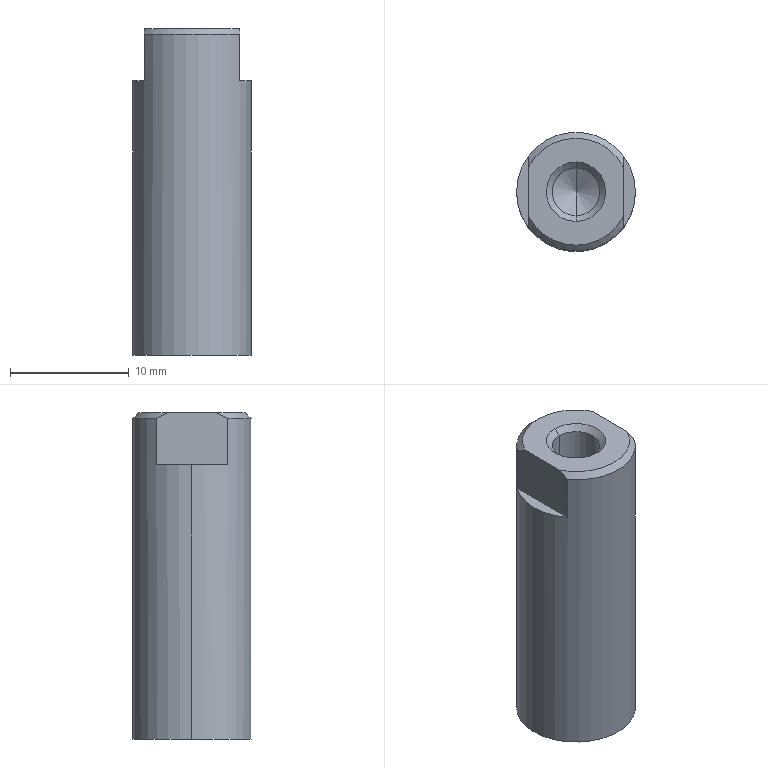Part | STEP file | CDQ2A20_15D_1_F7NV0 | 1 solid | 16 faces | box 10 x 10 x 27.5 mm | volume 2020 mm3 | cone 6 | plane 6 | cylinder 4 | commonest cylinder face diameters 4.02 x2 10 x2
STEP:
#1=CARTESIAN_POINT('',(0.,0.,0.));
#2=DIRECTION('',(0.,0.,1.));
#3=DIRECTION('',(1.,0.,0.));
#4=AXIS2_PLACEMENT_3D('',#1,#2,#3);
#5=CARTESIAN_POINT('',(0.,2.01,-3.));
#6=VERTEX_POINT('',#5);
#7=CARTESIAN_POINT('',(0.,-2.01,-3.));
#8=VERTEX_POINT('',#7);
#9=CARTESIAN_POINT('',(0.,0.,-3.));
#10=DIRECTION('',(0.,0.,1.));
#11=DIRECTION('',(0.,-1.,0.));
#12=AXIS2_PLACEMENT_3D('',#9,#10,#11);
#13=CIRCLE('',#12,2.01);
#14=CARTESIAN_POINT('',(0.,0.,995.84));
#15=DIRECTION('',(0.,0.,1.));
#16=DIRECTION('',(0.,-1.,0.));
#17=AXIS2_PLACEMENT_3D('',#14,#15,#16);
#18=CONICAL_SURFACE('',#17,1732.051,1.047);
#19=CARTESIAN_POINT('',(0.,-998.84));
#20=DIRECTION('',(1.,0.));
#21=VECTOR('',#20,1.);
#22=LINE('',#19,#21);
#23=(GEOMETRIC_REPRESENTATION_CONTEXT(2)PARAMETRIC_REPRESENTATION_CONTEXT()REPRESENTATION_CONTEXT('',''));
#24=DEFINITIONAL_REPRESENTATION('',(#22),#23);
#25=PCURVE('',#18,#24);
#26=CARTESIAN_POINT('',(0.,0.,-4.16));
#27=DIRECTION('',(0.,0.,1.));
#28=DIRECTION('',(0.,-1.,0.));
#29=AXIS2_PLACEMENT_3D('',#26,#27,#28);
#30=CYLINDRICAL_SURFACE('',#29,2.01);
#31=CARTESIAN_POINT('',(0.,1.16));
#32=DIRECTION('',(1.,0.));
#33=VECTOR('',#32,1.);
#34=LINE('',#31,#33);
#35=(GEOMETRIC_REPRESENTATION_CONTEXT(2)PARAMETRIC_REPRESENTATION_CONTEXT()REPRESENTATION_CONTEXT('',''));
#36=DEFINITIONAL_REPRESENTATION('',(#34),#35);
#37=PCURVE('',#30,#36);
#38=SURFACE_CURVE('',#13,(#25,#37),.PCURVE_S1.);
#39=EDGE_CURVE('',#6,#8,#38,.T.);
#40=ORIENTED_EDGE('',*,*,#39,.F.);
#41=CARTESIAN_POINT('',(0.,0.,-4.16));
#42=VERTEX_POINT('',#41);
#43=CARTESIAN_POINT('',(0.,0.,-4.16));
#44=DIRECTION('',(0.,0.866,0.5));
#45=VECTOR('',#44,1.);
#46=LINE('',#43,#45);
#47=CARTESIAN_POINT('',(3.142,-1000.));
#48=CARTESIAN_POINT('',(3.142,-999.982));
#49=CARTESIAN_POINT('',(3.142,-999.947));
#50=CARTESIAN_POINT('',(3.142,-999.895));
#51=CARTESIAN_POINT('',(3.142,-999.842));
#52=CARTESIAN_POINT('',(3.142,-999.789));
#53=CARTESIAN_POINT('',(3.142,-999.736));
#54=CARTESIAN_POINT('',(3.142,-999.684));
#55=CARTESIAN_POINT('',(3.142,-999.631));
#56=CARTESIAN_POINT('',(3.142,-999.578));
#57=CARTESIAN_POINT('',(3.142,-999.525));
#58=CARTESIAN_POINT('',(3.142,-999.473));
#59=CARTESIAN_POINT('',(3.142,-999.42));
#60=CARTESIAN_POINT('',(3.142,-999.367));
#61=CARTESIAN_POINT('',(3.142,-999.314));
#62=CARTESIAN_POINT('',(3.142,-999.262));
#63=CARTESIAN_POINT('',(3.142,-999.209));
#64=CARTESIAN_POINT('',(3.142,-999.156));
#65=CARTESIAN_POINT('',(3.142,-999.103));
#66=CARTESIAN_POINT('',(3.142,-999.051));
#67=CARTESIAN_POINT('',(3.142,-998.998));
#68=CARTESIAN_POINT('',(3.142,-998.945));
#69=CARTESIAN_POINT('',(3.142,-998.892));
#70=CARTESIAN_POINT('',(3.142,-998.857));
#71=CARTESIAN_POINT('',(3.142,-998.84));
#72=B_SPLINE_CURVE_WITH_KNOTS('',3,(#47,#48,#49,#50,#51,#52,#53,#54,#55,#56,#57,#58,#59,#60,#61,#62,#63,#64,#65,#66,#67,#68,#69,#70,#71),.UNSPECIFIED.,.F.,.F.,(4,1,1,1,1,1,1,1,1,1,1,1,1,1,1,1,1,1,1,1,1,1,4),(0.,0.1055,0.211,0.3165,0.422,0.5275,0.633,0.7385,0.844,0.9495,1.055,1.16,1.266,1.371,1.477,1.582,1.688,1.793,1.899,2.004,2.11,2.215,2.321),.QUASI_UNIFORM_KNOTS.);
#73=(GEOMETRIC_REPRESENTATION_CONTEXT(2)PARAMETRIC_REPRESENTATION_CONTEXT()REPRESENTATION_CONTEXT('',''));
#74=DEFINITIONAL_REPRESENTATION('',(#72),#73);
#75=PCURVE('',#18,#74);
#76=CARTESIAN_POINT('',(0.,0.,995.84));
#77=DIRECTION('',(0.,0.,1.));
#78=DIRECTION('',(0.,-1.,0.));
#79=AXIS2_PLACEMENT_3D('',#76,#77,#78);
#80=CONICAL_SURFACE('',#79,1732.051,1.047);
#81=CARTESIAN_POINT('',(3.142,-1000.));
#82=CARTESIAN_POINT('',(3.142,-999.982));
#83=CARTESIAN_POINT('',(3.142,-999.947));
#84=CARTESIAN_POINT('',(3.142,-999.895));
#85=CARTESIAN_POINT('',(3.142,-999.842));
#86=CARTESIAN_POINT('',(3.142,-999.789));
#87=CARTESIAN_POINT('',(3.142,-999.736));
#88=CARTESIAN_POINT('',(3.142,-999.684));
#89=CARTESIAN_POINT('',(3.142,-999.631));
#90=CARTESIAN_POINT('',(3.142,-999.578));
#91=CARTESIAN_POINT('',(3.142,-999.525));
#92=CARTESIAN_POINT('',(3.142,-999.473));
#93=CARTESIAN_POINT('',(3.142,-999.42));
#94=CARTESIAN_POINT('',(3.142,-999.367));
#95=CARTESIAN_POINT('',(3.142,-999.314));
#96=CARTESIAN_POINT('',(3.142,-999.262));
#97=CARTESIAN_POINT('',(3.142,-999.209));
#98=CARTESIAN_POINT('',(3.142,-999.156));
#99=CARTESIAN_POINT('',(3.142,-999.103));
#100=CARTESIAN_POINT('',(3.142,-999.051));
#101=CARTESIAN_POINT('',(3.142,-998.998));
#102=CARTESIAN_POINT('',(3.142,-998.945));
#103=CARTESIAN_POINT('',(3.142,-998.892));
#104=CARTESIAN_POINT('',(3.142,-998.857));
#105=CARTESIAN_POINT('',(3.142,-998.84));
#106=B_SPLINE_CURVE_WITH_KNOTS('',3,(#81,#82,#83,#84,#85,#86,#87,#88,#89,#90,#91,#92,#93,#94,#95,#96,#97,#98,#99,#100,#101,#102,#103,#104,#105),.UNSPECIFIED.,.F.,.F.,(4,1,1,1,1,1,1,1,1,1,1,1,1,1,1,1,1,1,1,1,1,1,4),(0.,0.1055,0.211,0.3165,0.422,0.5275,0.633,0.7385,0.844,0.9495,1.055,1.16,1.266,1.371,1.477,1.582,1.688,1.793,1.899,2.004,2.11,2.215,2.321),.QUASI_UNIFORM_KNOTS.);
#107=(GEOMETRIC_REPRESENTATION_CONTEXT(2)PARAMETRIC_REPRESENTATION_CONTEXT()REPRESENTATION_CONTEXT('',''));
#108=DEFINITIONAL_REPRESENTATION('',(#106),#107);
#109=PCURVE('',#80,#108);
#110=SURFACE_CURVE('',#46,(#75,#109),.PCURVE_S1.);
#111=EDGE_CURVE('',#42,#6,#110,.T.);
#112=ORIENTED_EDGE('',*,*,#111,.F.);
#113=CARTESIAN_POINT('',(0.,0.,-4.16));
#114=DIRECTION('',(0.,-0.866,0.5));
#115=VECTOR('',#114,1.);
#116=LINE('',#113,#115);
#117=CARTESIAN_POINT('',(6.283,-1000.));
#118=DIRECTION('',(0.,1.));
#119=VECTOR('',#118,1.);
#120=LINE('',#117,#119);
#121=(GEOMETRIC_REPRESENTATION_CONTEXT(2)PARAMETRIC_REPRESENTATION_CONTEXT()REPRESENTATION_CONTEXT('',''));
#122=DEFINITIONAL_REPRESENTATION('',(#120),#121);
#123=PCURVE('',#18,#122);
#124=CARTESIAN_POINT('',(0.,-1000.));
#125=DIRECTION('',(0.,1.));
#126=VECTOR('',#125,1.);
#127=LINE('',#124,#126);
#128=(GEOMETRIC_REPRESENTATION_CONTEXT(2)PARAMETRIC_REPRESENTATION_CONTEXT()REPRESENTATION_CONTEXT('',''));
#129=DEFINITIONAL_REPRESENTATION('',(#127),#128);
#130=PCURVE('',#80,#129);
#131=SURFACE_CURVE('',#116,(#123,#130),.PCURVE_S1.);
#132=EDGE_CURVE('',#42,#8,#131,.T.);
#133=ORIENTED_EDGE('',*,*,#132,.T.);
#134=EDGE_LOOP('',(#40,#112,#133));
#135=FACE_BOUND('',#134,.F.);
#136=ADVANCED_FACE('',(#135),#18,.F.);
#137=CARTESIAN_POINT('',(0.,-2.01,4.01));
#138=VERTEX_POINT('',#137);
#139=CARTESIAN_POINT('',(0.,-2.01,-4.16));
#140=DIRECTION('',(0.,0.,1.));
#141=VECTOR('',#140,1.);
#142=LINE('',#139,#141);
#143=CARTESIAN_POINT('',(6.283,0.));
#144=DIRECTION('',(0.,1.));
#145=VECTOR('',#144,1.);
#146=LINE('',#143,#145);
#147=(GEOMETRIC_REPRESENTATION_CONTEXT(2)PARAMETRIC_REPRESENTATION_CONTEXT()REPRESENTATION_CONTEXT('',''));
#148=DEFINITIONAL_REPRESENTATION('',(#146),#147);
#149=PCURVE('',#30,#148);
#150=CARTESIAN_POINT('',(0.,0.,-4.16));
#151=DIRECTION('',(0.,0.,1.));
#152=DIRECTION('',(0.,-1.,0.));
#153=AXIS2_PLACEMENT_3D('',#150,#151,#152);
#154=CYLINDRICAL_SURFACE('',#153,2.01);
#155=CARTESIAN_POINT('',(0.,0.));
#156=DIRECTION('',(0.,1.));
#157=VECTOR('',#156,1.);
#158=LINE('',#155,#157);
#159=(GEOMETRIC_REPRESENTATION_CONTEXT(2)PARAMETRIC_REPRESENTATION_CONTEXT()REPRESENTATION_CONTEXT('',''));
#160=DEFINITIONAL_REPRESENTATION('',(#158),#159);
#161=PCURVE('',#154,#160);
#162=SURFACE_CURVE('',#142,(#149,#161),.PCURVE_S1.);
#163=EDGE_CURVE('',#8,#138,#162,.T.);
#164=ORIENTED_EDGE('',*,*,#163,.T.);
#165=CARTESIAN_POINT('',(0.,2.01,4.01));
#166=VERTEX_POINT('',#165);
#167=CARTESIAN_POINT('',(0.,0.,4.01));
#168=DIRECTION('',(0.,0.,1.));
#169=DIRECTION('',(0.,-1.,0.));
#170=AXIS2_PLACEMENT_3D('',#167,#168,#169);
#171=CIRCLE('',#170,2.01);
#172=CARTESIAN_POINT('',(0.,8.17));
#173=DIRECTION('',(1.,0.));
#174=VECTOR('',#173,1.);
#175=LINE('',#172,#174);
#176=(GEOMETRIC_REPRESENTATION_CONTEXT(2)PARAMETRIC_REPRESENTATION_CONTEXT()REPRESENTATION_CONTEXT('',''));
#177=DEFINITIONAL_REPRESENTATION('',(#175),#176);
#178=PCURVE('',#30,#177);
#179=CARTESIAN_POINT('',(0.,0.,4.01));
#180=DIRECTION('',(0.,0.,1.));
#181=DIRECTION('',(0.,-1.,0.));
#182=AXIS2_PLACEMENT_3D('',#179,#180,#181);
#183=CONICAL_SURFACE('',#182,2.01,0.7854);
#184=CARTESIAN_POINT('',(0.,0.));
#185=DIRECTION('',(1.,0.));
#186=VECTOR('',#185,1.);
#187=LINE('',#184,#186);
#188=(GEOMETRIC_REPRESENTATION_CONTEXT(2)PARAMETRIC_REPRESENTATION_CONTEXT()REPRESENTATION_CONTEXT('',''));
#189=DEFINITIONAL_REPRESENTATION('',(#187),#188);
#190=PCURVE('',#183,#189);
#191=SURFACE_CURVE('',#171,(#178,#190),.PCURVE_S1.);
#192=EDGE_CURVE('',#166,#138,#191,.T.);
#193=ORIENTED_EDGE('',*,*,#192,.F.);
#194=CARTESIAN_POINT('',(0.,2.01,-4.16));
#195=DIRECTION('',(0.,0.,1.));
#196=VECTOR('',#195,1.);
#197=LINE('',#194,#196);
#198=CARTESIAN_POINT('',(3.142,0.));
#199=DIRECTION('',(0.,1.));
#200=VECTOR('',#199,1.);
#201=LINE('',#198,#200);
#202=(GEOMETRIC_REPRESENTATION_CONTEXT(2)PARAMETRIC_REPRESENTATION_CONTEXT()REPRESENTATION_CONTEXT('',''));
#203=DEFINITIONAL_REPRESENTATION('',(#201),#202);
#204=PCURVE('',#30,#203);
#205=CARTESIAN_POINT('',(3.142,0.));
#206=DIRECTION('',(0.,1.));
#207=VECTOR('',#206,1.);
#208=LINE('',#205,#207);
#209=(GEOMETRIC_REPRESENTATION_CONTEXT(2)PARAMETRIC_REPRESENTATION_CONTEXT()REPRESENTATION_CONTEXT('',''));
#210=DEFINITIONAL_REPRESENTATION('',(#208),#209);
#211=PCURVE('',#154,#210);
#212=SURFACE_CURVE('',#197,(#204,#211),.PCURVE_S1.);
#213=EDGE_CURVE('',#6,#166,#212,.T.);
#214=ORIENTED_EDGE('',*,*,#213,.F.);
#215=ORIENTED_EDGE('',*,*,#39,.T.);
#216=EDGE_LOOP('',(#164,#193,#214,#215));
#217=FACE_BOUND('',#216,.F.);
#218=ADVANCED_FACE('',(#217),#30,.F.);
#219=CARTESIAN_POINT('',(0.,-2.5,4.5));
#220=VERTEX_POINT('',#219);
#221=CARTESIAN_POINT('',(0.,-2.01,4.01));
#222=DIRECTION('',(0.,-0.7071,0.7071));
#223=VECTOR('',#222,1.);
#224=LINE('',#221,#223);
#225=CARTESIAN_POINT('',(6.283,0.));
#226=DIRECTION('',(0.,1.));
#227=VECTOR('',#226,1.);
#228=LINE('',#225,#227);
#229=(GEOMETRIC_REPRESENTATION_CONTEXT(2)PARAMETRIC_REPRESENTATION_CONTEXT()REPRESENTATION_CONTEXT('',''));
#230=DEFINITIONAL_REPRESENTATION('',(#228),#229);
#231=PCURVE('',#183,#230);
#232=CARTESIAN_POINT('',(0.,0.,4.01));
#233=DIRECTION('',(0.,0.,1.));
#234=DIRECTION('',(0.,-1.,0.));
#235=AXIS2_PLACEMENT_3D('',#232,#233,#234);
#236=CONICAL_SURFACE('',#235,2.01,0.7854);
#237=CARTESIAN_POINT('',(0.,0.));
#238=DIRECTION('',(0.,1.));
#239=VECTOR('',#238,1.);
#240=LINE('',#237,#239);
#241=(GEOMETRIC_REPRESENTATION_CONTEXT(2)PARAMETRIC_REPRESENTATION_CONTEXT()REPRESENTATION_CONTEXT('',''));
#242=DEFINITIONAL_REPRESENTATION('',(#240),#241);
#243=PCURVE('',#236,#242);
#244=SURFACE_CURVE('',#224,(#231,#243),.PCURVE_S1.);
#245=EDGE_CURVE('',#138,#220,#244,.T.);
#246=ORIENTED_EDGE('',*,*,#245,.T.);
#247=CARTESIAN_POINT('',(0.,2.5,4.5));
#248=VERTEX_POINT('',#247);
#249=CARTESIAN_POINT('',(0.,0.,4.5));
#250=DIRECTION('',(0.,0.,1.));
#251=DIRECTION('',(-1.,0.,0.));
#252=AXIS2_PLACEMENT_3D('',#249,#250,#251);
#253=CIRCLE('',#252,2.5);
#254=CARTESIAN_POINT('',(-1.571,0.49));
#255=DIRECTION('',(1.,0.));
#256=VECTOR('',#255,1.);
#257=LINE('',#254,#256);
#258=(GEOMETRIC_REPRESENTATION_CONTEXT(2)PARAMETRIC_REPRESENTATION_CONTEXT()REPRESENTATION_CONTEXT('',''));
#259=DEFINITIONAL_REPRESENTATION('',(#257),#258);
#260=PCURVE('',#183,#259);
#261=CARTESIAN_POINT('',(0.,0.,4.5));
#262=DIRECTION('',(0.,0.,-1.));
#263=DIRECTION('',(-1.,0.,0.));
#264=AXIS2_PLACEMENT_3D('',#261,#262,#263);
#265=PLANE('',#264);
#266=CARTESIAN_POINT('',(2.5,0.));
#267=CARTESIAN_POINT('',(2.5,-4.33));
#268=CARTESIAN_POINT('',(-1.25,-2.165));
#269=CARTESIAN_POINT('',(-5.,0.));
#270=CARTESIAN_POINT('',(-1.25,2.165));
#271=CARTESIAN_POINT('',(2.5,4.33));
#272=CARTESIAN_POINT('',(2.5,0.));
#273=(BOUNDED_CURVE()B_SPLINE_CURVE(2,(#266,#267,#268,#269,#270,#271,#272),.UNSPECIFIED.,.T.,.F.)B_SPLINE_CURVE_WITH_KNOTS((1,2,2,2,2,1),(-2.094,0.,2.094,4.189,6.283,8.378),.UNSPECIFIED.)CURVE()GEOMETRIC_REPRESENTATION_ITEM()RATIONAL_B_SPLINE_CURVE((1.,0.5,1.,0.5,1.,0.5,1.))REPRESENTATION_ITEM(''));
#274=(GEOMETRIC_REPRESENTATION_CONTEXT(2)PARAMETRIC_REPRESENTATION_CONTEXT()REPRESENTATION_CONTEXT('',''));
#275=DEFINITIONAL_REPRESENTATION('',(#273),#274);
#276=PCURVE('',#265,#275);
#277=SURFACE_CURVE('',#253,(#260,#276),.PCURVE_S1.);
#278=EDGE_CURVE('',#248,#220,#277,.T.);
#279=ORIENTED_EDGE('',*,*,#278,.F.);
#280=CARTESIAN_POINT('',(0.,2.01,4.01));
#281=DIRECTION('',(0.,0.7071,0.7071));
#282=VECTOR('',#281,1.);
#283=LINE('',#280,#282);
#284=CARTESIAN_POINT('',(3.142,0.));
#285=DIRECTION('',(0.,1.));
#286=VECTOR('',#285,1.);
#287=LINE('',#284,#286);
#288=(GEOMETRIC_REPRESENTATION_CONTEXT(2)PARAMETRIC_REPRESENTATION_CONTEXT()REPRESENTATION_CONTEXT('',''));
#289=DEFINITIONAL_REPRESENTATION('',(#287),#288);
#290=PCURVE('',#183,#289);
#291=CARTESIAN_POINT('',(3.142,0.));
#292=DIRECTION('',(0.,1.));
#293=VECTOR('',#292,1.);
#294=LINE('',#291,#293);
#295=(GEOMETRIC_REPRESENTATION_CONTEXT(2)PARAMETRIC_REPRESENTATION_CONTEXT()REPRESENTATION_CONTEXT('',''));
#296=DEFINITIONAL_REPRESENTATION('',(#294),#295);
#297=PCURVE('',#236,#296);
#298=SURFACE_CURVE('',#283,(#290,#297),.PCURVE_S1.);
#299=EDGE_CURVE('',#166,#248,#298,.T.);
#300=ORIENTED_EDGE('',*,*,#299,.F.);
#301=ORIENTED_EDGE('',*,*,#192,.T.);
#302=EDGE_LOOP('',(#246,#279,#300,#301));
#303=FACE_BOUND('',#302,.F.);
#304=ADVANCED_FACE('',(#303),#183,.F.);
#305=CARTESIAN_POINT('',(5.,0.,-23.));
#306=VERTEX_POINT('',#305);
#307=CARTESIAN_POINT('',(-5.,0.,-23.));
#308=VERTEX_POINT('',#307);
#309=CARTESIAN_POINT('',(0.,0.,-23.));
#310=DIRECTION('',(0.,0.,1.));
#311=DIRECTION('',(1.,0.,0.));
#312=AXIS2_PLACEMENT_3D('',#309,#310,#311);
#313=CIRCLE('',#312,5.);
#314=CARTESIAN_POINT('',(0.,0.,-23.));
#315=DIRECTION('',(0.,0.,1.));
#316=DIRECTION('',(1.,0.,0.));
#317=AXIS2_PLACEMENT_3D('',#314,#315,#316);
#318=CYLINDRICAL_SURFACE('',#317,5.);
#319=CARTESIAN_POINT('',(0.,0.));
#320=DIRECTION('',(1.,0.));
#321=VECTOR('',#320,1.);
#322=LINE('',#319,#321);
#323=(GEOMETRIC_REPRESENTATION_CONTEXT(2)PARAMETRIC_REPRESENTATION_CONTEXT()REPRESENTATION_CONTEXT('',''));
#324=DEFINITIONAL_REPRESENTATION('',(#322),#323);
#325=PCURVE('',#318,#324);
#326=CARTESIAN_POINT('',(0.,5.,-23.));
#327=DIRECTION('',(0.,0.,1.));
#328=DIRECTION('',(1.,0.,0.));
#329=AXIS2_PLACEMENT_3D('',#326,#327,#328);
#330=PLANE('',#329);
#331=CARTESIAN_POINT('',(0.,-5.));
#332=DIRECTION('',(1.,0.));
#333=AXIS2_PLACEMENT_2D('',#331,#332);
#334=CIRCLE('',#333,5.);
#335=(GEOMETRIC_REPRESENTATION_CONTEXT(2)PARAMETRIC_REPRESENTATION_CONTEXT()REPRESENTATION_CONTEXT('',''));
#336=DEFINITIONAL_REPRESENTATION('',(#334),#335);
#337=PCURVE('',#330,#336);
#338=SURFACE_CURVE('',#313,(#325,#337),.PCURVE_S1.);
#339=EDGE_CURVE('',#306,#308,#338,.T.);
#340=ORIENTED_EDGE('',*,*,#339,.T.);
#341=CARTESIAN_POINT('',(-5.,0.,0.1));
#342=VERTEX_POINT('',#341);
#343=CARTESIAN_POINT('',(-5.,0.,-23.));
#344=DIRECTION('',(0.,0.,1.));
#345=VECTOR('',#344,1.);
#346=LINE('',#343,#345);
#347=CARTESIAN_POINT('',(3.142,0.));
#348=DIRECTION('',(0.,1.));
#349=VECTOR('',#348,1.);
#350=LINE('',#347,#349);
#351=(GEOMETRIC_REPRESENTATION_CONTEXT(2)PARAMETRIC_REPRESENTATION_CONTEXT()REPRESENTATION_CONTEXT('',''));
#352=DEFINITIONAL_REPRESENTATION('',(#350),#351);
#353=PCURVE('',#318,#352);
#354=CARTESIAN_POINT('',(0.,0.,-23.));
#355=DIRECTION('',(0.,0.,1.));
#356=DIRECTION('',(1.,0.,0.));
#357=AXIS2_PLACEMENT_3D('',#354,#355,#356);
#358=CYLINDRICAL_SURFACE('',#357,5.);
#359=CARTESIAN_POINT('',(3.142,0.));
#360=DIRECTION('',(0.,1.));
#361=VECTOR('',#360,1.);
#362=LINE('',#359,#361);
#363=(GEOMETRIC_REPRESENTATION_CONTEXT(2)PARAMETRIC_REPRESENTATION_CONTEXT()REPRESENTATION_CONTEXT('',''));
#364=DEFINITIONAL_REPRESENTATION('',(#362),#363);
#365=PCURVE('',#358,#364);
#366=SURFACE_CURVE('',#346,(#353,#365),.PCURVE_S1.);
#367=EDGE_CURVE('',#308,#342,#366,.T.);
#368=ORIENTED_EDGE('',*,*,#367,.T.);
#369=CARTESIAN_POINT('',(-4.,3.,0.1));
#370=VERTEX_POINT('',#369);
#371=CARTESIAN_POINT('',(0.,0.,0.1));
#372=DIRECTION('',(0.,0.,1.));
#373=DIRECTION('',(1.,0.,0.));
#374=AXIS2_PLACEMENT_3D('',#371,#372,#373);
#375=CIRCLE('',#374,5.);
#376=CARTESIAN_POINT('',(0.,23.1));
#377=DIRECTION('',(1.,0.));
#378=VECTOR('',#377,1.);
#379=LINE('',#376,#378);
#380=(GEOMETRIC_REPRESENTATION_CONTEXT(2)PARAMETRIC_REPRESENTATION_CONTEXT()REPRESENTATION_CONTEXT('',''));
#381=DEFINITIONAL_REPRESENTATION('',(#379),#380);
#382=PCURVE('',#318,#381);
#383=CARTESIAN_POINT('',(0.,0.,0.1));
#384=DIRECTION('',(0.,0.,1.));
#385=DIRECTION('',(1.,0.,0.));
#386=AXIS2_PLACEMENT_3D('',#383,#384,#385);
#387=PLANE('',#386);
#388=CARTESIAN_POINT('',(0.,0.));
#389=DIRECTION('',(1.,0.));
#390=AXIS2_PLACEMENT_2D('',#388,#389);
#391=CIRCLE('',#390,5.);
#392=(GEOMETRIC_REPRESENTATION_CONTEXT(2)PARAMETRIC_REPRESENTATION_CONTEXT()REPRESENTATION_CONTEXT('',''));
#393=DEFINITIONAL_REPRESENTATION('',(#391),#392);
#394=PCURVE('',#387,#393);
#395=SURFACE_CURVE('',#375,(#382,#394),.PCURVE_S1.);
#396=EDGE_CURVE('',#370,#342,#395,.T.);
#397=ORIENTED_EDGE('',*,*,#396,.F.);
#398=CARTESIAN_POINT('',(-4.,3.,4.));
#399=VERTEX_POINT('',#398);
#400=CARTESIAN_POINT('',(-4.,3.,-23.));
#401=DIRECTION('',(0.,0.,1.));
#402=VECTOR('',#401,1.);
#403=LINE('',#400,#402);
#404=CARTESIAN_POINT('',(2.498,0.));
#405=DIRECTION('',(0.,1.));
#406=VECTOR('',#405,1.);
#407=LINE('',#404,#406);
#408=(GEOMETRIC_REPRESENTATION_CONTEXT(2)PARAMETRIC_REPRESENTATION_CONTEXT()REPRESENTATION_CONTEXT('',''));
#409=DEFINITIONAL_REPRESENTATION('',(#407),#408);
#410=PCURVE('',#318,#409);
#411=CARTESIAN_POINT('',(-4.,-7.,0.1));
#412=DIRECTION('',(1.,0.,0.));
#413=DIRECTION('',(0.,0.,-1.));
#414=AXIS2_PLACEMENT_3D('',#411,#412,#413);
#415=PLANE('',#414);
#416=CARTESIAN_POINT('',(23.1,10.));
#417=DIRECTION('',(-1.,0.));
#418=VECTOR('',#417,1.);
#419=LINE('',#416,#418);
#420=(GEOMETRIC_REPRESENTATION_CONTEXT(2)PARAMETRIC_REPRESENTATION_CONTEXT()REPRESENTATION_CONTEXT('',''));
#421=DEFINITIONAL_REPRESENTATION('',(#419),#420);
#422=PCURVE('',#415,#421);
#423=SURFACE_CURVE('',#403,(#410,#422),.PCURVE_S1.);
#424=EDGE_CURVE('',#370,#399,#423,.T.);
#425=ORIENTED_EDGE('',*,*,#424,.T.);
#426=CARTESIAN_POINT('',(4.,3.,4.));
#427=VERTEX_POINT('',#426);
#428=CARTESIAN_POINT('',(0.,0.,4.));
#429=DIRECTION('',(0.,0.,1.));
#430=DIRECTION('',(1.,0.,0.));
#431=AXIS2_PLACEMENT_3D('',#428,#429,#430);
#432=CIRCLE('',#431,5.);
#433=CARTESIAN_POINT('',(0.,27.));
#434=DIRECTION('',(1.,0.));
#435=VECTOR('',#434,1.);
#436=LINE('',#433,#435);
#437=(GEOMETRIC_REPRESENTATION_CONTEXT(2)PARAMETRIC_REPRESENTATION_CONTEXT()REPRESENTATION_CONTEXT('',''));
#438=DEFINITIONAL_REPRESENTATION('',(#436),#437);
#439=PCURVE('',#318,#438);
#440=CARTESIAN_POINT('',(0.,0.,4.));
#441=DIRECTION('',(0.,0.,-1.));
#442=DIRECTION('',(-1.,0.,0.));
#443=AXIS2_PLACEMENT_3D('',#440,#441,#442);
#444=CONICAL_SURFACE('',#443,5.,0.7854);
#445=CARTESIAN_POINT('',(3.142,0.));
#446=DIRECTION('',(-1.,0.));
#447=VECTOR('',#446,1.);
#448=LINE('',#445,#447);
#449=(GEOMETRIC_REPRESENTATION_CONTEXT(2)PARAMETRIC_REPRESENTATION_CONTEXT()REPRESENTATION_CONTEXT('',''));
#450=DEFINITIONAL_REPRESENTATION('',(#448),#449);
#451=PCURVE('',#444,#450);
#452=SURFACE_CURVE('',#432,(#439,#451),.PCURVE_S1.);
#453=EDGE_CURVE('',#427,#399,#452,.T.);
#454=ORIENTED_EDGE('',*,*,#453,.F.);
#455=CARTESIAN_POINT('',(4.,3.,0.1));
#456=VERTEX_POINT('',#455);
#457=CARTESIAN_POINT('',(4.,3.,-23.));
#458=DIRECTION('',(0.,0.,-1.));
#459=VECTOR('',#458,1.);
#460=LINE('',#457,#459);
#461=CARTESIAN_POINT('',(0.6435,0.));
#462=DIRECTION('',(0.,-1.));
#463=VECTOR('',#462,1.);
#464=LINE('',#461,#463);
#465=(GEOMETRIC_REPRESENTATION_CONTEXT(2)PARAMETRIC_REPRESENTATION_CONTEXT()REPRESENTATION_CONTEXT('',''));
#466=DEFINITIONAL_REPRESENTATION('',(#464),#465);
#467=PCURVE('',#318,#466);
#468=CARTESIAN_POINT('',(4.,7.,0.1));
#469=DIRECTION('',(-1.,0.,0.));
#470=DIRECTION('',(0.,0.,1.));
#471=AXIS2_PLACEMENT_3D('',#468,#469,#470);
#472=PLANE('',#471);
#473=CARTESIAN_POINT('',(-23.1,-4.));
#474=DIRECTION('',(-1.,0.));
#475=VECTOR('',#474,1.);
#476=LINE('',#473,#475);
#477=(GEOMETRIC_REPRESENTATION_CONTEXT(2)PARAMETRIC_REPRESENTATION_CONTEXT()REPRESENTATION_CONTEXT('',''));
#478=DEFINITIONAL_REPRESENTATION('',(#476),#477);
#479=PCURVE('',#472,#478);
#480=SURFACE_CURVE('',#460,(#467,#479),.PCURVE_S1.);
#481=EDGE_CURVE('',#427,#456,#480,.T.);
#482=ORIENTED_EDGE('',*,*,#481,.T.);
#483=CARTESIAN_POINT('',(5.,0.,0.1));
#484=VERTEX_POINT('',#483);
#485=CARTESIAN_POINT('',(0.,0.,0.1));
#486=DIRECTION('',(0.,0.,1.));
#487=DIRECTION('',(1.,0.,0.));
#488=AXIS2_PLACEMENT_3D('',#485,#486,#487);
#489=CIRCLE('',#488,5.);
#490=CARTESIAN_POINT('',(0.,23.1));
#491=DIRECTION('',(1.,0.));
#492=VECTOR('',#491,1.);
#493=LINE('',#490,#492);
#494=(GEOMETRIC_REPRESENTATION_CONTEXT(2)PARAMETRIC_REPRESENTATION_CONTEXT()REPRESENTATION_CONTEXT('',''));
#495=DEFINITIONAL_REPRESENTATION('',(#493),#494);
#496=PCURVE('',#318,#495);
#497=CARTESIAN_POINT('',(0.,0.,0.1));
#498=DIRECTION('',(0.,0.,1.));
#499=DIRECTION('',(1.,0.,0.));
#500=AXIS2_PLACEMENT_3D('',#497,#498,#499);
#501=PLANE('',#500);
#502=CARTESIAN_POINT('',(0.,0.));
#503=DIRECTION('',(1.,0.));
#504=AXIS2_PLACEMENT_2D('',#502,#503);
#505=CIRCLE('',#504,5.);
#506=(GEOMETRIC_REPRESENTATION_CONTEXT(2)PARAMETRIC_REPRESENTATION_CONTEXT()REPRESENTATION_CONTEXT('',''));
#507=DEFINITIONAL_REPRESENTATION('',(#505),#506);
#508=PCURVE('',#501,#507);
#509=SURFACE_CURVE('',#489,(#496,#508),.PCURVE_S1.);
#510=EDGE_CURVE('',#484,#456,#509,.T.);
#511=ORIENTED_EDGE('',*,*,#510,.F.);
#512=CARTESIAN_POINT('',(5.,0.,-23.));
#513=DIRECTION('',(0.,0.,1.));
#514=VECTOR('',#513,1.);
#515=LINE('',#512,#514);
#516=CARTESIAN_POINT('',(0.,0.));
#517=DIRECTION('',(0.,1.));
#518=VECTOR('',#517,1.);
#519=LINE('',#516,#518);
#520=(GEOMETRIC_REPRESENTATION_CONTEXT(2)PARAMETRIC_REPRESENTATION_CONTEXT()REPRESENTATION_CONTEXT('',''));
#521=DEFINITIONAL_REPRESENTATION('',(#519),#520);
#522=PCURVE('',#318,#521);
#523=CARTESIAN_POINT('',(6.283,0.));
#524=DIRECTION('',(0.,1.));
#525=VECTOR('',#524,1.);
#526=LINE('',#523,#525);
#527=(GEOMETRIC_REPRESENTATION_CONTEXT(2)PARAMETRIC_REPRESENTATION_CONTEXT()REPRESENTATION_CONTEXT('',''));
#528=DEFINITIONAL_REPRESENTATION('',(#526),#527);
#529=PCURVE('',#358,#528);
#530=SURFACE_CURVE('',#515,(#522,#529),.PCURVE_S1.);
#531=EDGE_CURVE('',#306,#484,#530,.T.);
#532=ORIENTED_EDGE('',*,*,#531,.F.);
#533=EDGE_LOOP('',(#340,#368,#397,#425,#454,#482,#511,#532));
#534=FACE_BOUND('',#533,.T.);
#535=ADVANCED_FACE('',(#534),#318,.T.);
#536=CARTESIAN_POINT('',(-4.,-2.062,4.5));
#537=VERTEX_POINT('',#536);
#538=CARTESIAN_POINT('',(4.,-2.062,4.5));
#539=VERTEX_POINT('',#538);
#540=CARTESIAN_POINT('',(0.,0.,4.5));
#541=DIRECTION('',(0.,0.,1.));
#542=DIRECTION('',(1.,0.,0.));
#543=AXIS2_PLACEMENT_3D('',#540,#541,#542);
#544=CIRCLE('',#543,4.5);
#545=CARTESIAN_POINT('',(-4.5,0.));
#546=CARTESIAN_POINT('',(-4.5,7.794));
#547=CARTESIAN_POINT('',(2.25,3.897));
#548=CARTESIAN_POINT('',(9.,0.));
#549=CARTESIAN_POINT('',(2.25,-3.897));
#550=CARTESIAN_POINT('',(-4.5,-7.794));
#551=CARTESIAN_POINT('',(-4.5,0.));
#552=(BOUNDED_CURVE()B_SPLINE_CURVE(2,(#545,#546,#547,#548,#549,#550,#551),.UNSPECIFIED.,.T.,.F.)B_SPLINE_CURVE_WITH_KNOTS((1,2,2,2,2,1),(-2.094,0.,2.094,4.189,6.283,8.378),.UNSPECIFIED.)CURVE()GEOMETRIC_REPRESENTATION_ITEM()RATIONAL_B_SPLINE_CURVE((1.,0.5,1.,0.5,1.,0.5,1.))REPRESENTATION_ITEM(''));
#553=(GEOMETRIC_REPRESENTATION_CONTEXT(2)PARAMETRIC_REPRESENTATION_CONTEXT()REPRESENTATION_CONTEXT('',''));
#554=DEFINITIONAL_REPRESENTATION('',(#552),#553);
#555=PCURVE('',#265,#554);
#556=CARTESIAN_POINT('',(0.,0.,4.));
#557=DIRECTION('',(0.,0.,-1.));
#558=DIRECTION('',(-1.,0.,0.));
#559=AXIS2_PLACEMENT_3D('',#556,#557,#558);
#560=CONICAL_SURFACE('',#559,5.,0.7854);
#561=CARTESIAN_POINT('',(9.425,-0.5));
#562=DIRECTION('',(-1.,0.));
#563=VECTOR('',#562,1.);
#564=LINE('',#561,#563);
#565=(GEOMETRIC_REPRESENTATION_CONTEXT(2)PARAMETRIC_REPRESENTATION_CONTEXT()REPRESENTATION_CONTEXT('',''));
#566=DEFINITIONAL_REPRESENTATION('',(#564),#565);
#567=PCURVE('',#560,#566);
#568=SURFACE_CURVE('',#544,(#555,#567),.PCURVE_S1.);
#569=EDGE_CURVE('',#537,#539,#568,.T.);
#570=ORIENTED_EDGE('',*,*,#569,.T.);
#571=CARTESIAN_POINT('',(4.,2.062,4.5));
#572=VERTEX_POINT('',#571);
#573=CARTESIAN_POINT('',(4.,7.,4.5));
#574=DIRECTION('',(0.,-1.,0.));
#575=VECTOR('',#574,1.);
#576=LINE('',#573,#575);
#577=CARTESIAN_POINT('',(-4.,7.));
#578=DIRECTION('',(0.,-1.));
#579=VECTOR('',#578,1.);
#580=LINE('',#577,#579);
#581=(GEOMETRIC_REPRESENTATION_CONTEXT(2)PARAMETRIC_REPRESENTATION_CONTEXT()REPRESENTATION_CONTEXT('',''));
#582=DEFINITIONAL_REPRESENTATION('',(#580),#581);
#583=PCURVE('',#265,#582);
#584=CARTESIAN_POINT('',(4.4,0.));
#585=DIRECTION('',(0.,-1.));
#586=VECTOR('',#585,1.);
#587=LINE('',#584,#586);
#588=(GEOMETRIC_REPRESENTATION_CONTEXT(2)PARAMETRIC_REPRESENTATION_CONTEXT()REPRESENTATION_CONTEXT('',''));
#589=DEFINITIONAL_REPRESENTATION('',(#587),#588);
#590=PCURVE('',#472,#589);
#591=SURFACE_CURVE('',#576,(#583,#590),.PCURVE_S1.);
#592=EDGE_CURVE('',#572,#539,#591,.T.);
#593=ORIENTED_EDGE('',*,*,#592,.F.);
#594=CARTESIAN_POINT('',(-4.,2.062,4.5));
#595=VERTEX_POINT('',#594);
#596=CARTESIAN_POINT('',(0.,0.,4.5));
#597=DIRECTION('',(0.,0.,1.));
#598=DIRECTION('',(1.,0.,0.));
#599=AXIS2_PLACEMENT_3D('',#596,#597,#598);
#600=CIRCLE('',#599,4.5);
#601=CARTESIAN_POINT('',(-4.5,0.));
#602=CARTESIAN_POINT('',(-4.5,7.794));
#603=CARTESIAN_POINT('',(2.25,3.897));
#604=CARTESIAN_POINT('',(9.,0.));
#605=CARTESIAN_POINT('',(2.25,-3.897));
#606=CARTESIAN_POINT('',(-4.5,-7.794));
#607=CARTESIAN_POINT('',(-4.5,0.));
#608=(BOUNDED_CURVE()B_SPLINE_CURVE(2,(#601,#602,#603,#604,#605,#606,#607),.UNSPECIFIED.,.T.,.F.)B_SPLINE_CURVE_WITH_KNOTS((1,2,2,2,2,1),(-2.094,0.,2.094,4.189,6.283,8.378),.UNSPECIFIED.)CURVE()GEOMETRIC_REPRESENTATION_ITEM()RATIONAL_B_SPLINE_CURVE((1.,0.5,1.,0.5,1.,0.5,1.))REPRESENTATION_ITEM(''));
#609=(GEOMETRIC_REPRESENTATION_CONTEXT(2)PARAMETRIC_REPRESENTATION_CONTEXT()REPRESENTATION_CONTEXT('',''));
#610=DEFINITIONAL_REPRESENTATION('',(#608),#609);
#611=PCURVE('',#265,#610);
#612=CARTESIAN_POINT('',(3.142,-0.5));
#613=DIRECTION('',(-1.,0.));
#614=VECTOR('',#613,1.);
#615=LINE('',#612,#614);
#616=(GEOMETRIC_REPRESENTATION_CONTEXT(2)PARAMETRIC_REPRESENTATION_CONTEXT()REPRESENTATION_CONTEXT('',''));
#617=DEFINITIONAL_REPRESENTATION('',(#615),#616);
#618=PCURVE('',#444,#617);
#619=SURFACE_CURVE('',#600,(#611,#618),.PCURVE_S1.);
#620=EDGE_CURVE('',#572,#595,#619,.T.);
#621=ORIENTED_EDGE('',*,*,#620,.T.);
#622=CARTESIAN_POINT('',(-4.,-7.,4.5));
#623=DIRECTION('',(0.,1.,0.));
#624=VECTOR('',#623,1.);
#625=LINE('',#622,#624);
#626=CARTESIAN_POINT('',(4.,-7.));
#627=DIRECTION('',(0.,1.));
#628=VECTOR('',#627,1.);
#629=LINE('',#626,#628);
#630=(GEOMETRIC_REPRESENTATION_CONTEXT(2)PARAMETRIC_REPRESENTATION_CONTEXT()REPRESENTATION_CONTEXT('',''));
#631=DEFINITIONAL_REPRESENTATION('',(#629),#630);
#632=PCURVE('',#265,#631);
#633=CARTESIAN_POINT('',(-4.4,0.));
#634=DIRECTION('',(0.,1.));
#635=VECTOR('',#634,1.);
#636=LINE('',#633,#635);
#637=(GEOMETRIC_REPRESENTATION_CONTEXT(2)PARAMETRIC_REPRESENTATION_CONTEXT()REPRESENTATION_CONTEXT('',''));
#638=DEFINITIONAL_REPRESENTATION('',(#636),#637);
#639=PCURVE('',#415,#638);
#640=SURFACE_CURVE('',#625,(#632,#639),.PCURVE_S1.);
#641=EDGE_CURVE('',#537,#595,#640,.T.);
#642=ORIENTED_EDGE('',*,*,#641,.F.);
#643=EDGE_LOOP('',(#570,#593,#621,#642));
#644=FACE_BOUND('',#643,.T.);
#645=CARTESIAN_POINT('',(0.,0.,4.5));
#646=DIRECTION('',(0.,0.,1.));
#647=DIRECTION('',(-1.,0.,0.));
#648=AXIS2_PLACEMENT_3D('',#645,#646,#647);
#649=CIRCLE('',#648,2.5);
#650=CARTESIAN_POINT('',(2.5,0.));
#651=CARTESIAN_POINT('',(2.5,-4.33));
#652=CARTESIAN_POINT('',(-1.25,-2.165));
#653=CARTESIAN_POINT('',(-5.,0.));
#654=CARTESIAN_POINT('',(-1.25,2.165));
#655=CARTESIAN_POINT('',(2.5,4.33));
#656=CARTESIAN_POINT('',(2.5,0.));
#657=(BOUNDED_CURVE()B_SPLINE_CURVE(2,(#650,#651,#652,#653,#654,#655,#656),.UNSPECIFIED.,.T.,.F.)B_SPLINE_CURVE_WITH_KNOTS((1,2,2,2,2,1),(-2.094,0.,2.094,4.189,6.283,8.378),.UNSPECIFIED.)CURVE()GEOMETRIC_REPRESENTATION_ITEM()RATIONAL_B_SPLINE_CURVE((1.,0.5,1.,0.5,1.,0.5,1.))REPRESENTATION_ITEM(''));
#658=(GEOMETRIC_REPRESENTATION_CONTEXT(2)PARAMETRIC_REPRESENTATION_CONTEXT()REPRESENTATION_CONTEXT('',''));
#659=DEFINITIONAL_REPRESENTATION('',(#657),#658);
#660=PCURVE('',#265,#659);
#661=CARTESIAN_POINT('',(-1.571,0.49));
#662=DIRECTION('',(1.,0.));
#663=VECTOR('',#662,1.);
#664=LINE('',#661,#663);
#665=(GEOMETRIC_REPRESENTATION_CONTEXT(2)PARAMETRIC_REPRESENTATION_CONTEXT()REPRESENTATION_CONTEXT('',''));
#666=DEFINITIONAL_REPRESENTATION('',(#664),#665);
#667=PCURVE('',#236,#666);
#668=SURFACE_CURVE('',#649,(#660,#667),.PCURVE_S1.);
#669=EDGE_CURVE('',#220,#248,#668,.T.);
#670=ORIENTED_EDGE('',*,*,#669,.F.);
#671=ORIENTED_EDGE('',*,*,#278,.F.);
#672=EDGE_LOOP('',(#670,#671));
#673=FACE_BOUND('',#672,.T.);
#674=ADVANCED_FACE('',(#644,#673),#265,.F.);
#675=CARTESIAN_POINT('',(-4.,-3.,4.));
#676=VERTEX_POINT('',#675);
#677=CARTESIAN_POINT('',(4.,-3.,4.));
#678=VERTEX_POINT('',#677);
#679=CARTESIAN_POINT('',(0.,0.,4.));
#680=DIRECTION('',(0.,0.,1.));
#681=DIRECTION('',(1.,0.,0.));
#682=AXIS2_PLACEMENT_3D('',#679,#680,#681);
#683=CIRCLE('',#682,5.);
#684=CARTESIAN_POINT('',(9.425,0.));
#685=DIRECTION('',(-1.,0.));
#686=VECTOR('',#685,1.);
#687=LINE('',#684,#686);
#688=(GEOMETRIC_REPRESENTATION_CONTEXT(2)PARAMETRIC_REPRESENTATION_CONTEXT()REPRESENTATION_CONTEXT('',''));
#689=DEFINITIONAL_REPRESENTATION('',(#687),#688);
#690=PCURVE('',#560,#689);
#691=CARTESIAN_POINT('',(0.,27.));
#692=DIRECTION('',(1.,0.));
#693=VECTOR('',#692,1.);
#694=LINE('',#691,#693);
#695=(GEOMETRIC_REPRESENTATION_CONTEXT(2)PARAMETRIC_REPRESENTATION_CONTEXT()REPRESENTATION_CONTEXT('',''));
#696=DEFINITIONAL_REPRESENTATION('',(#694),#695);
#697=PCURVE('',#358,#696);
#698=SURFACE_CURVE('',#683,(#690,#697),.PCURVE_S1.);
#699=EDGE_CURVE('',#676,#678,#698,.T.);
#700=ORIENTED_EDGE('',*,*,#699,.T.);
#701=CARTESIAN_POINT('',(4.,-3.,4.));
#702=CARTESIAN_POINT('',(4.,-2.695,4.183));
#703=CARTESIAN_POINT('',(4.,-2.384,4.352));
#704=CARTESIAN_POINT('',(4.,-2.062,4.5));
#705=B_SPLINE_CURVE_WITH_KNOTS('',3,(#701,#702,#703,#704),.UNSPECIFIED.,.F.,.F.,(4,4),(0.009434,0.0105),.PIECEWISE_BEZIER_KNOTS.);
#706=CARTESIAN_POINT('',(3.785,0.));
#707=CARTESIAN_POINT('',(3.783,-0.008314));
#708=CARTESIAN_POINT('',(3.778,-0.02489));
#709=CARTESIAN_POINT('',(3.772,-0.04957));
#710=CARTESIAN_POINT('',(3.765,-0.07408));
#711=CARTESIAN_POINT('',(3.758,-0.09841));
#712=CARTESIAN_POINT('',(3.751,-0.1225));
#713=CARTESIAN_POINT('',(3.744,-0.1465));
#714=CARTESIAN_POINT('',(3.737,-0.1703));
#715=CARTESIAN_POINT('',(3.729,-0.1938));
#716=CARTESIAN_POINT('',(3.722,-0.2172));
#717=CARTESIAN_POINT('',(3.714,-0.2403));
#718=CARTESIAN_POINT('',(3.707,-0.2632));
#719=CARTESIAN_POINT('',(3.699,-0.286));
#720=CARTESIAN_POINT('',(3.692,-0.3084));
#721=CARTESIAN_POINT('',(3.684,-0.3307));
#722=CARTESIAN_POINT('',(3.676,-0.3527));
#723=CARTESIAN_POINT('',(3.668,-0.3745));
#724=CARTESIAN_POINT('',(3.66,-0.3961));
#725=CARTESIAN_POINT('',(3.651,-0.4174));
#726=CARTESIAN_POINT('',(3.643,-0.4385));
#727=CARTESIAN_POINT('',(3.635,-0.4593));
#728=CARTESIAN_POINT('',(3.626,-0.4798));
#729=CARTESIAN_POINT('',(3.62,-0.4933));
#730=CARTESIAN_POINT('',(3.617,-0.5));
#731=B_SPLINE_CURVE_WITH_KNOTS('',3,(#706,#707,#708,#709,#710,#711,#712,#713,#714,#715,#716,#717,#718,#719,#720,#721,#722,#723,#724,#725,#726,#727,#728,#729,#730),.UNSPECIFIED.,.F.,.F.,(4,1,1,1,1,1,1,1,1,1,1,1,1,1,1,1,1,1,1,1,1,1,4),(0.009434,0.009483,0.009531,0.009579,0.009628,0.009676,0.009724,0.009773,0.009821,0.00987,0.009918,0.009966,0.01001,0.01006,0.01011,0.01016,0.01021,0.01026,0.0103,0.01035,0.0104,0.01045,0.0105),.QUASI_UNIFORM_KNOTS.);
#732=(GEOMETRIC_REPRESENTATION_CONTEXT(2)PARAMETRIC_REPRESENTATION_CONTEXT()REPRESENTATION_CONTEXT('',''));
#733=DEFINITIONAL_REPRESENTATION('',(#731),#732);
#734=PCURVE('',#560,#733);
#735=CARTESIAN_POINT('',(3.9,-10.));
#736=CARTESIAN_POINT('',(4.083,-9.695));
#737=CARTESIAN_POINT('',(4.252,-9.384));
#738=CARTESIAN_POINT('',(4.4,-9.062));
#739=B_SPLINE_CURVE_WITH_KNOTS('',3,(#735,#736,#737,#738),.UNSPECIFIED.,.F.,.F.,(4,4),(0.009434,0.0105),.PIECEWISE_BEZIER_KNOTS.);
#740=(GEOMETRIC_REPRESENTATION_CONTEXT(2)PARAMETRIC_REPRESENTATION_CONTEXT()REPRESENTATION_CONTEXT('',''));
#741=DEFINITIONAL_REPRESENTATION('',(#739),#740);
#742=PCURVE('',#472,#741);
#743=SURFACE_CURVE('',#705,(#734,#742),.PCURVE_S1.);
#744=EDGE_CURVE('',#678,#539,#743,.T.);
#745=ORIENTED_EDGE('',*,*,#744,.T.);
#746=ORIENTED_EDGE('',*,*,#569,.F.);
#747=CARTESIAN_POINT('',(-4.,-2.062,4.5));
#748=CARTESIAN_POINT('',(-4.,-2.385,4.352));
#749=CARTESIAN_POINT('',(-4.,-2.696,4.182));
#750=CARTESIAN_POINT('',(-4.,-3.,4.));
#751=B_SPLINE_CURVE_WITH_KNOTS('',3,(#747,#748,#749,#750),.UNSPECIFIED.,.F.,.F.,(4,4),(0.01478,0.01585),.PIECEWISE_BEZIER_KNOTS.);
#752=CARTESIAN_POINT('',(5.807,-0.5));
#753=CARTESIAN_POINT('',(5.804,-0.4933));
#754=CARTESIAN_POINT('',(5.799,-0.4797));
#755=CARTESIAN_POINT('',(5.79,-0.4591));
#756=CARTESIAN_POINT('',(5.782,-0.4383));
#757=CARTESIAN_POINT('',(5.773,-0.4172));
#758=CARTESIAN_POINT('',(5.765,-0.3958));
#759=CARTESIAN_POINT('',(5.757,-0.3742));
#760=CARTESIAN_POINT('',(5.749,-0.3524));
#761=CARTESIAN_POINT('',(5.741,-0.3303));
#762=CARTESIAN_POINT('',(5.733,-0.308));
#763=CARTESIAN_POINT('',(5.725,-0.2855));
#764=CARTESIAN_POINT('',(5.718,-0.2628));
#765=CARTESIAN_POINT('',(5.71,-0.2399));
#766=CARTESIAN_POINT('',(5.703,-0.2167));
#767=CARTESIAN_POINT('',(5.695,-0.1934));
#768=CARTESIAN_POINT('',(5.688,-0.1699));
#769=CARTESIAN_POINT('',(5.681,-0.1462));
#770=CARTESIAN_POINT('',(5.674,-0.1222));
#771=CARTESIAN_POINT('',(5.667,-0.09815));
#772=CARTESIAN_POINT('',(5.66,-0.07388));
#773=CARTESIAN_POINT('',(5.653,-0.04943));
#774=CARTESIAN_POINT('',(5.646,-0.02481));
#775=CARTESIAN_POINT('',(5.642,-0.008288));
#776=CARTESIAN_POINT('',(5.64,0.));
#777=B_SPLINE_CURVE_WITH_KNOTS('',3,(#752,#753,#754,#755,#756,#757,#758,#759,#760,#761,#762,#763,#764,#765,#766,#767,#768,#769,#770,#771,#772,#773,#774,#775,#776),.UNSPECIFIED.,.F.,.F.,(4,1,1,1,1,1,1,1,1,1,1,1,1,1,1,1,1,1,1,1,1,1,4),(0.01478,0.01482,0.01487,0.01492,0.01497,0.01502,0.01507,0.01512,0.01517,0.01522,0.01526,0.01531,0.01536,0.01541,0.01546,0.01551,0.01556,0.01561,0.01566,0.0157,0.01575,0.0158,0.01585),.QUASI_UNIFORM_KNOTS.);
#778=(GEOMETRIC_REPRESENTATION_CONTEXT(2)PARAMETRIC_REPRESENTATION_CONTEXT()REPRESENTATION_CONTEXT('',''));
#779=DEFINITIONAL_REPRESENTATION('',(#777),#778);
#780=PCURVE('',#560,#779);
#781=CARTESIAN_POINT('',(-4.4,4.938));
#782=CARTESIAN_POINT('',(-4.252,4.615));
#783=CARTESIAN_POINT('',(-4.082,4.304));
#784=CARTESIAN_POINT('',(-3.9,4.));
#785=B_SPLINE_CURVE_WITH_KNOTS('',3,(#781,#782,#783,#784),.UNSPECIFIED.,.F.,.F.,(4,4),(0.01478,0.01585),.PIECEWISE_BEZIER_KNOTS.);
#786=(GEOMETRIC_REPRESENTATION_CONTEXT(2)PARAMETRIC_REPRESENTATION_CONTEXT()REPRESENTATION_CONTEXT('',''));
#787=DEFINITIONAL_REPRESENTATION('',(#785),#786);
#788=PCURVE('',#415,#787);
#789=SURFACE_CURVE('',#751,(#780,#788),.PCURVE_S1.);
#790=EDGE_CURVE('',#537,#676,#789,.T.);
#791=ORIENTED_EDGE('',*,*,#790,.T.);
#792=EDGE_LOOP('',(#700,#745,#746,#791));
#793=FACE_BOUND('',#792,.T.);
#794=ADVANCED_FACE('',(#793),#560,.T.);
#795=ORIENTED_EDGE('',*,*,#620,.F.);
#796=CARTESIAN_POINT('',(4.,2.062,4.5));
#797=CARTESIAN_POINT('',(4.,2.385,4.352));
#798=CARTESIAN_POINT('',(4.,2.696,4.182));
#799=CARTESIAN_POINT('',(4.,3.,4.));
#800=B_SPLINE_CURVE_WITH_KNOTS('',3,(#796,#797,#798,#799),.UNSPECIFIED.,.F.,.F.,(4,4),(0.01478,0.01585),.PIECEWISE_BEZIER_KNOTS.);
#801=CARTESIAN_POINT('',(2.666,-0.5));
#802=CARTESIAN_POINT('',(2.663,-0.4933));
#803=CARTESIAN_POINT('',(2.657,-0.4797));
#804=CARTESIAN_POINT('',(2.648,-0.4591));
#805=CARTESIAN_POINT('',(2.64,-0.4383));
#806=CARTESIAN_POINT('',(2.632,-0.4172));
#807=CARTESIAN_POINT('',(2.623,-0.3958));
#808=CARTESIAN_POINT('',(2.615,-0.3742));
#809=CARTESIAN_POINT('',(2.607,-0.3524));
#810=CARTESIAN_POINT('',(2.599,-0.3303));
#811=CARTESIAN_POINT('',(2.592,-0.308));
#812=CARTESIAN_POINT('',(2.584,-0.2855));
#813=CARTESIAN_POINT('',(2.576,-0.2628));
#814=CARTESIAN_POINT('',(2.569,-0.2399));
#815=CARTESIAN_POINT('',(2.561,-0.2167));
#816=CARTESIAN_POINT('',(2.554,-0.1934));
#817=CARTESIAN_POINT('',(2.547,-0.1699));
#818=CARTESIAN_POINT('',(2.539,-0.1462));
#819=CARTESIAN_POINT('',(2.532,-0.1222));
#820=CARTESIAN_POINT('',(2.525,-0.09815));
#821=CARTESIAN_POINT('',(2.518,-0.07388));
#822=CARTESIAN_POINT('',(2.512,-0.04943));
#823=CARTESIAN_POINT('',(2.505,-0.02481));
#824=CARTESIAN_POINT('',(2.5,-0.008288));
#825=CARTESIAN_POINT('',(2.498,0.));
#826=B_SPLINE_CURVE_WITH_KNOTS('',3,(#801,#802,#803,#804,#805,#806,#807,#808,#809,#810,#811,#812,#813,#814,#815,#816,#817,#818,#819,#820,#821,#822,#823,#824,#825),.UNSPECIFIED.,.F.,.F.,(4,1,1,1,1,1,1,1,1,1,1,1,1,1,1,1,1,1,1,1,1,1,4),(0.01478,0.01482,0.01487,0.01492,0.01497,0.01502,0.01507,0.01512,0.01517,0.01522,0.01526,0.01531,0.01536,0.01541,0.01546,0.01551,0.01556,0.01561,0.01566,0.0157,0.01575,0.0158,0.01585),.QUASI_UNIFORM_KNOTS.);
#827=(GEOMETRIC_REPRESENTATION_CONTEXT(2)PARAMETRIC_REPRESENTATION_CONTEXT()REPRESENTATION_CONTEXT('',''));
#828=DEFINITIONAL_REPRESENTATION('',(#826),#827);
#829=PCURVE('',#444,#828);
#830=CARTESIAN_POINT('',(4.4,-4.938));
#831=CARTESIAN_POINT('',(4.252,-4.615));
#832=CARTESIAN_POINT('',(4.082,-4.304));
#833=CARTESIAN_POINT('',(3.9,-4.));
#834=B_SPLINE_CURVE_WITH_KNOTS('',3,(#830,#831,#832,#833),.UNSPECIFIED.,.F.,.F.,(4,4),(0.01478,0.01585),.PIECEWISE_BEZIER_KNOTS.);
#835=(GEOMETRIC_REPRESENTATION_CONTEXT(2)PARAMETRIC_REPRESENTATION_CONTEXT()REPRESENTATION_CONTEXT('',''));
#836=DEFINITIONAL_REPRESENTATION('',(#834),#835);
#837=PCURVE('',#472,#836);
#838=SURFACE_CURVE('',#800,(#829,#837),.PCURVE_S1.);
#839=EDGE_CURVE('',#572,#427,#838,.T.);
#840=ORIENTED_EDGE('',*,*,#839,.T.);
#841=ORIENTED_EDGE('',*,*,#453,.T.);
#842=CARTESIAN_POINT('',(-4.,3.,4.));
#843=CARTESIAN_POINT('',(-4.,2.695,4.183));
#844=CARTESIAN_POINT('',(-4.,2.384,4.352));
#845=CARTESIAN_POINT('',(-4.,2.062,4.5));
#846=B_SPLINE_CURVE_WITH_KNOTS('',3,(#842,#843,#844,#845),.UNSPECIFIED.,.F.,.F.,(4,4),(0.009434,0.0105),.PIECEWISE_BEZIER_KNOTS.);
#847=CARTESIAN_POINT('',(0.6435,0.));
#848=CARTESIAN_POINT('',(0.6413,-0.008314));
#849=CARTESIAN_POINT('',(0.6368,-0.02489));
#850=CARTESIAN_POINT('',(0.6301,-0.04957));
#851=CARTESIAN_POINT('',(0.6232,-0.07408));
#852=CARTESIAN_POINT('',(0.6163,-0.09841));
#853=CARTESIAN_POINT('',(0.6092,-0.1225));
#854=CARTESIAN_POINT('',(0.6021,-0.1465));
#855=CARTESIAN_POINT('',(0.5949,-0.1703));
#856=CARTESIAN_POINT('',(0.5877,-0.1938));
#857=CARTESIAN_POINT('',(0.5803,-0.2172));
#858=CARTESIAN_POINT('',(0.5728,-0.2403));
#859=CARTESIAN_POINT('',(0.5653,-0.2632));
#860=CARTESIAN_POINT('',(0.5576,-0.286));
#861=CARTESIAN_POINT('',(0.5499,-0.3084));
#862=CARTESIAN_POINT('',(0.5421,-0.3307));
#863=CARTESIAN_POINT('',(0.5342,-0.3527));
#864=CARTESIAN_POINT('',(0.5261,-0.3745));
#865=CARTESIAN_POINT('',(0.518,-0.3961));
#866=CARTESIAN_POINT('',(0.5098,-0.4174));
#867=CARTESIAN_POINT('',(0.5015,-0.4385));
#868=CARTESIAN_POINT('',(0.493,-0.4593));
#869=CARTESIAN_POINT('',(0.4845,-0.4798));
#870=CARTESIAN_POINT('',(0.4788,-0.4933));
#871=CARTESIAN_POINT('',(0.4759,-0.5));
#872=B_SPLINE_CURVE_WITH_KNOTS('',3,(#847,#848,#849,#850,#851,#852,#853,#854,#855,#856,#857,#858,#859,#860,#861,#862,#863,#864,#865,#866,#867,#868,#869,#870,#871),.UNSPECIFIED.,.F.,.F.,(4,1,1,1,1,1,1,1,1,1,1,1,1,1,1,1,1,1,1,1,1,1,4),(0.009434,0.009483,0.009531,0.009579,0.009628,0.009676,0.009724,0.009773,0.009821,0.00987,0.009918,0.009966,0.01001,0.01006,0.01011,0.01016,0.01021,0.01026,0.0103,0.01035,0.0104,0.01045,0.0105),.QUASI_UNIFORM_KNOTS.);
#873=(GEOMETRIC_REPRESENTATION_CONTEXT(2)PARAMETRIC_REPRESENTATION_CONTEXT()REPRESENTATION_CONTEXT('',''));
#874=DEFINITIONAL_REPRESENTATION('',(#872),#873);
#875=PCURVE('',#444,#874);
#876=CARTESIAN_POINT('',(-3.9,10.));
#877=CARTESIAN_POINT('',(-4.083,9.695));
#878=CARTESIAN_POINT('',(-4.252,9.384));
#879=CARTESIAN_POINT('',(-4.4,9.062));
#880=B_SPLINE_CURVE_WITH_KNOTS('',3,(#876,#877,#878,#879),.UNSPECIFIED.,.F.,.F.,(4,4),(0.009434,0.0105),.PIECEWISE_BEZIER_KNOTS.);
#881=(GEOMETRIC_REPRESENTATION_CONTEXT(2)PARAMETRIC_REPRESENTATION_CONTEXT()REPRESENTATION_CONTEXT('',''));
#882=DEFINITIONAL_REPRESENTATION('',(#880),#881);
#883=PCURVE('',#415,#882);
#884=SURFACE_CURVE('',#846,(#875,#883),.PCURVE_S1.);
#885=EDGE_CURVE('',#399,#595,#884,.T.);
#886=ORIENTED_EDGE('',*,*,#885,.T.);
#887=EDGE_LOOP('',(#795,#840,#841,#886));
#888=FACE_BOUND('',#887,.T.);
#889=ADVANCED_FACE('',(#888),#444,.T.);
#890=ORIENTED_EDGE('',*,*,#367,.F.);
#891=CARTESIAN_POINT('',(0.,0.,-23.));
#892=DIRECTION('',(0.,0.,1.));
#893=DIRECTION('',(1.,0.,0.));
#894=AXIS2_PLACEMENT_3D('',#891,#892,#893);
#895=CIRCLE('',#894,5.);
#896=CARTESIAN_POINT('',(0.,0.));
#897=DIRECTION('',(1.,0.));
#898=VECTOR('',#897,1.);
#899=LINE('',#896,#898);
#900=(GEOMETRIC_REPRESENTATION_CONTEXT(2)PARAMETRIC_REPRESENTATION_CONTEXT()REPRESENTATION_CONTEXT('',''));
#901=DEFINITIONAL_REPRESENTATION('',(#899),#900);
#902=PCURVE('',#358,#901);
#903=CARTESIAN_POINT('',(0.,-5.));
#904=DIRECTION('',(1.,0.));
#905=AXIS2_PLACEMENT_2D('',#903,#904);
#906=CIRCLE('',#905,5.);
#907=(GEOMETRIC_REPRESENTATION_CONTEXT(2)PARAMETRIC_REPRESENTATION_CONTEXT()REPRESENTATION_CONTEXT('',''));
#908=DEFINITIONAL_REPRESENTATION('',(#906),#907);
#909=PCURVE('',#330,#908);
#910=SURFACE_CURVE('',#895,(#902,#909),.PCURVE_S1.);
#911=EDGE_CURVE('',#308,#306,#910,.T.);
#912=ORIENTED_EDGE('',*,*,#911,.T.);
#913=ORIENTED_EDGE('',*,*,#531,.T.);
#914=CARTESIAN_POINT('',(4.,-3.,0.1));
#915=VERTEX_POINT('',#914);
#916=CARTESIAN_POINT('',(0.,0.,0.1));
#917=DIRECTION('',(0.,0.,1.));
#918=DIRECTION('',(1.,0.,0.));
#919=AXIS2_PLACEMENT_3D('',#916,#917,#918);
#920=CIRCLE('',#919,5.);
#921=CARTESIAN_POINT('',(0.,23.1));
#922=DIRECTION('',(1.,0.));
#923=VECTOR('',#922,1.);
#924=LINE('',#921,#923);
#925=(GEOMETRIC_REPRESENTATION_CONTEXT(2)PARAMETRIC_REPRESENTATION_CONTEXT()REPRESENTATION_CONTEXT('',''));
#926=DEFINITIONAL_REPRESENTATION('',(#924),#925);
#927=PCURVE('',#358,#926);
#928=CARTESIAN_POINT('',(0.,0.));
#929=DIRECTION('',(1.,0.));
#930=AXIS2_PLACEMENT_2D('',#928,#929);
#931=CIRCLE('',#930,5.);
#932=(GEOMETRIC_REPRESENTATION_CONTEXT(2)PARAMETRIC_REPRESENTATION_CONTEXT()REPRESENTATION_CONTEXT('',''));
#933=DEFINITIONAL_REPRESENTATION('',(#931),#932);
#934=PCURVE('',#501,#933);
#935=SURFACE_CURVE('',#920,(#927,#934),.PCURVE_S1.);
#936=EDGE_CURVE('',#915,#484,#935,.T.);
#937=ORIENTED_EDGE('',*,*,#936,.F.);
#938=CARTESIAN_POINT('',(4.,-3.,-23.));
#939=DIRECTION('',(0.,0.,1.));
#940=VECTOR('',#939,1.);
#941=LINE('',#938,#940);
#942=CARTESIAN_POINT('',(5.64,0.));
#943=DIRECTION('',(0.,1.));
#944=VECTOR('',#943,1.);
#945=LINE('',#942,#944);
#946=(GEOMETRIC_REPRESENTATION_CONTEXT(2)PARAMETRIC_REPRESENTATION_CONTEXT()REPRESENTATION_CONTEXT('',''));
#947=DEFINITIONAL_REPRESENTATION('',(#945),#946);
#948=PCURVE('',#358,#947);
#949=CARTESIAN_POINT('',(-23.1,-10.));
#950=DIRECTION('',(1.,0.));
#951=VECTOR('',#950,1.);
#952=LINE('',#949,#951);
#953=(GEOMETRIC_REPRESENTATION_CONTEXT(2)PARAMETRIC_REPRESENTATION_CONTEXT()REPRESENTATION_CONTEXT('',''));
#954=DEFINITIONAL_REPRESENTATION('',(#952),#953);
#955=PCURVE('',#472,#954);
#956=SURFACE_CURVE('',#941,(#948,#955),.PCURVE_S1.);
#957=EDGE_CURVE('',#915,#678,#956,.T.);
#958=ORIENTED_EDGE('',*,*,#957,.T.);
#959=ORIENTED_EDGE('',*,*,#699,.F.);
#960=CARTESIAN_POINT('',(-4.,-3.,0.1));
#961=VERTEX_POINT('',#960);
#962=CARTESIAN_POINT('',(-4.,-3.,-23.));
#963=DIRECTION('',(0.,0.,-1.));
#964=VECTOR('',#963,1.);
#965=LINE('',#962,#964);
#966=CARTESIAN_POINT('',(3.785,0.));
#967=DIRECTION('',(0.,-1.));
#968=VECTOR('',#967,1.);
#969=LINE('',#966,#968);
#970=(GEOMETRIC_REPRESENTATION_CONTEXT(2)PARAMETRIC_REPRESENTATION_CONTEXT()REPRESENTATION_CONTEXT('',''));
#971=DEFINITIONAL_REPRESENTATION('',(#969),#970);
#972=PCURVE('',#358,#971);
#973=CARTESIAN_POINT('',(23.1,4.));
#974=DIRECTION('',(1.,0.));
#975=VECTOR('',#974,1.);
#976=LINE('',#973,#975);
#977=(GEOMETRIC_REPRESENTATION_CONTEXT(2)PARAMETRIC_REPRESENTATION_CONTEXT()REPRESENTATION_CONTEXT('',''));
#978=DEFINITIONAL_REPRESENTATION('',(#976),#977);
#979=PCURVE('',#415,#978);
#980=SURFACE_CURVE('',#965,(#972,#979),.PCURVE_S1.);
#981=EDGE_CURVE('',#676,#961,#980,.T.);
#982=ORIENTED_EDGE('',*,*,#981,.T.);
#983=CARTESIAN_POINT('',(0.,0.,0.1));
#984=DIRECTION('',(0.,0.,1.));
#985=DIRECTION('',(1.,0.,0.));
#986=AXIS2_PLACEMENT_3D('',#983,#984,#985);
#987=CIRCLE('',#986,5.);
#988=CARTESIAN_POINT('',(0.,23.1));
#989=DIRECTION('',(1.,0.));
#990=VECTOR('',#989,1.);
#991=LINE('',#988,#990);
#992=(GEOMETRIC_REPRESENTATION_CONTEXT(2)PARAMETRIC_REPRESENTATION_CONTEXT()REPRESENTATION_CONTEXT('',''));
#993=DEFINITIONAL_REPRESENTATION('',(#991),#992);
#994=PCURVE('',#358,#993);
#995=CARTESIAN_POINT('',(0.,0.));
#996=DIRECTION('',(1.,0.));
#997=AXIS2_PLACEMENT_2D('',#995,#996);
#998=CIRCLE('',#997,5.);
#999=(GEOMETRIC_REPRESENTATION_CONTEXT(2)PARAMETRIC_REPRESENTATION_CONTEXT()REPRESENTATION_CONTEXT('',''));
#1000=DEFINITIONAL_REPRESENTATION('',(#998),#999);
#1001=PCURVE('',#387,#1000);
#1002=SURFACE_CURVE('',#987,(#994,#1001),.PCURVE_S1.);
#1003=EDGE_CURVE('',#342,#961,#1002,.T.);
#1004=ORIENTED_EDGE('',*,*,#1003,.F.);
#1005=EDGE_LOOP('',(#890,#912,#913,#937,#958,#959,#982,#1004));
#1006=FACE_BOUND('',#1005,.T.);
#1007=ADVANCED_FACE('',(#1006),#358,.T.);
#1008=ORIENTED_EDGE('',*,*,#339,.F.);
#1009=ORIENTED_EDGE('',*,*,#911,.F.);
#1010=EDGE_LOOP('',(#1008,#1009));
#1011=FACE_BOUND('',#1010,.T.);
#1012=ADVANCED_FACE('',(#1011),#330,.F.);
#1013=ORIENTED_EDGE('',*,*,#936,.T.);
#1014=ORIENTED_EDGE('',*,*,#510,.T.);
#1015=CARTESIAN_POINT('',(4.,7.,0.1));
#1016=DIRECTION('',(0.,-1.,0.));
#1017=VECTOR('',#1016,1.);
#1018=LINE('',#1015,#1017);
#1019=CARTESIAN_POINT('',(4.,7.));
#1020=DIRECTION('',(0.,-1.));
#1021=VECTOR('',#1020,1.);
#1022=LINE('',#1019,#1021);
#1023=(GEOMETRIC_REPRESENTATION_CONTEXT(2)PARAMETRIC_REPRESENTATION_CONTEXT()REPRESENTATION_CONTEXT('',''));
#1024=DEFINITIONAL_REPRESENTATION('',(#1022),#1023);
#1025=PCURVE('',#501,#1024);
#1026=CARTESIAN_POINT('',(0.,0.));
#1027=DIRECTION('',(0.,-1.));
#1028=VECTOR('',#1027,1.);
#1029=LINE('',#1026,#1028);
#1030=(GEOMETRIC_REPRESENTATION_CONTEXT(2)PARAMETRIC_REPRESENTATION_CONTEXT()REPRESENTATION_CONTEXT('',''));
#1031=DEFINITIONAL_REPRESENTATION('',(#1029),#1030);
#1032=PCURVE('',#472,#1031);
#1033=SURFACE_CURVE('',#1018,(#1025,#1032),.PCURVE_S1.);
#1034=EDGE_CURVE('',#456,#915,#1033,.T.);
#1035=ORIENTED_EDGE('',*,*,#1034,.T.);
#1036=EDGE_LOOP('',(#1013,#1014,#1035));
#1037=FACE_BOUND('',#1036,.T.);
#1038=ADVANCED_FACE('',(#1037),#501,.T.);
#1039=ORIENTED_EDGE('',*,*,#957,.F.);
#1040=ORIENTED_EDGE('',*,*,#1034,.F.);
#1041=ORIENTED_EDGE('',*,*,#481,.F.);
#1042=ORIENTED_EDGE('',*,*,#839,.F.);
#1043=ORIENTED_EDGE('',*,*,#592,.T.);
#1044=ORIENTED_EDGE('',*,*,#744,.F.);
#1045=EDGE_LOOP('',(#1039,#1040,#1041,#1042,#1043,#1044));
#1046=FACE_BOUND('',#1045,.T.);
#1047=ADVANCED_FACE('',(#1046),#472,.F.);
#1048=ORIENTED_EDGE('',*,*,#424,.F.);
#1049=CARTESIAN_POINT('',(-4.,-7.,0.1));
#1050=DIRECTION('',(0.,1.,0.));
#1051=VECTOR('',#1050,1.);
#1052=LINE('',#1049,#1051);
#1053=CARTESIAN_POINT('',(0.,0.));
#1054=DIRECTION('',(0.,1.));
#1055=VECTOR('',#1054,1.);
#1056=LINE('',#1053,#1055);
#1057=(GEOMETRIC_REPRESENTATION_CONTEXT(2)PARAMETRIC_REPRESENTATION_CONTEXT()REPRESENTATION_CONTEXT('',''));
#1058=DEFINITIONAL_REPRESENTATION('',(#1056),#1057);
#1059=PCURVE('',#415,#1058);
#1060=CARTESIAN_POINT('',(-4.,-7.));
#1061=DIRECTION('',(0.,1.));
#1062=VECTOR('',#1061,1.);
#1063=LINE('',#1060,#1062);
#1064=(GEOMETRIC_REPRESENTATION_CONTEXT(2)PARAMETRIC_REPRESENTATION_CONTEXT()REPRESENTATION_CONTEXT('',''));
#1065=DEFINITIONAL_REPRESENTATION('',(#1063),#1064);
#1066=PCURVE('',#387,#1065);
#1067=SURFACE_CURVE('',#1052,(#1059,#1066),.PCURVE_S1.);
#1068=EDGE_CURVE('',#961,#370,#1067,.T.);
#1069=ORIENTED_EDGE('',*,*,#1068,.F.);
#1070=ORIENTED_EDGE('',*,*,#981,.F.);
#1071=ORIENTED_EDGE('',*,*,#790,.F.);
#1072=ORIENTED_EDGE('',*,*,#641,.T.);
#1073=ORIENTED_EDGE('',*,*,#885,.F.);
#1074=EDGE_LOOP('',(#1048,#1069,#1070,#1071,#1072,#1073));
#1075=FACE_BOUND('',#1074,.T.);
#1076=ADVANCED_FACE('',(#1075),#415,.F.);
#1077=ORIENTED_EDGE('',*,*,#396,.T.);
#1078=ORIENTED_EDGE('',*,*,#1003,.T.);
#1079=ORIENTED_EDGE('',*,*,#1068,.T.);
#1080=EDGE_LOOP('',(#1077,#1078,#1079));
#1081=FACE_BOUND('',#1080,.T.);
#1082=ADVANCED_FACE('',(#1081),#387,.T.);
#1083=ORIENTED_EDGE('',*,*,#669,.F.);
#1084=ORIENTED_EDGE('',*,*,#245,.F.);
#1085=CARTESIAN_POINT('',(0.,0.,4.01));
#1086=DIRECTION('',(0.,0.,1.));
#1087=DIRECTION('',(0.,-1.,0.));
#1088=AXIS2_PLACEMENT_3D('',#1085,#1086,#1087);
#1089=CIRCLE('',#1088,2.01);
#1090=CARTESIAN_POINT('',(0.,0.));
#1091=DIRECTION('',(1.,0.));
#1092=VECTOR('',#1091,1.);
#1093=LINE('',#1090,#1092);
#1094=(GEOMETRIC_REPRESENTATION_CONTEXT(2)PARAMETRIC_REPRESENTATION_CONTEXT()REPRESENTATION_CONTEXT('',''));
#1095=DEFINITIONAL_REPRESENTATION('',(#1093),#1094);
#1096=PCURVE('',#236,#1095);
#1097=CARTESIAN_POINT('',(0.,8.17));
#1098=DIRECTION('',(1.,0.));
#1099=VECTOR('',#1098,1.);
#1100=LINE('',#1097,#1099);
#1101=(GEOMETRIC_REPRESENTATION_CONTEXT(2)PARAMETRIC_REPRESENTATION_CONTEXT()REPRESENTATION_CONTEXT('',''));
#1102=DEFINITIONAL_REPRESENTATION('',(#1100),#1101);
#1103=PCURVE('',#154,#1102);
#1104=SURFACE_CURVE('',#1089,(#1096,#1103),.PCURVE_S1.);
#1105=EDGE_CURVE('',#138,#166,#1104,.T.);
#1106=ORIENTED_EDGE('',*,*,#1105,.T.);
#1107=ORIENTED_EDGE('',*,*,#299,.T.);
#1108=EDGE_LOOP('',(#1083,#1084,#1106,#1107));
#1109=FACE_BOUND('',#1108,.F.);
#1110=ADVANCED_FACE('',(#1109),#236,.F.);
#1111=ORIENTED_EDGE('',*,*,#1105,.F.);
#1112=ORIENTED_EDGE('',*,*,#163,.F.);
#1113=CARTESIAN_POINT('',(0.,0.,-3.));
#1114=DIRECTION('',(0.,0.,1.));
#1115=DIRECTION('',(0.,-1.,0.));
#1116=AXIS2_PLACEMENT_3D('',#1113,#1114,#1115);
#1117=CIRCLE('',#1116,2.01);
#1118=CARTESIAN_POINT('',(0.,1.16));
#1119=DIRECTION('',(1.,0.));
#1120=VECTOR('',#1119,1.);
#1121=LINE('',#1118,#1120);
#1122=(GEOMETRIC_REPRESENTATION_CONTEXT(2)PARAMETRIC_REPRESENTATION_CONTEXT()REPRESENTATION_CONTEXT('',''));
#1123=DEFINITIONAL_REPRESENTATION('',(#1121),#1122);
#1124=PCURVE('',#154,#1123);
#1125=CARTESIAN_POINT('',(0.,-998.84));
#1126=DIRECTION('',(1.,0.));
#1127=VECTOR('',#1126,1.);
#1128=LINE('',#1125,#1127);
#1129=(GEOMETRIC_REPRESENTATION_CONTEXT(2)PARAMETRIC_REPRESENTATION_CONTEXT()REPRESENTATION_CONTEXT('',''));
#1130=DEFINITIONAL_REPRESENTATION('',(#1128),#1129);
#1131=PCURVE('',#80,#1130);
#1132=SURFACE_CURVE('',#1117,(#1124,#1131),.PCURVE_S1.);
#1133=EDGE_CURVE('',#8,#6,#1132,.T.);
#1134=ORIENTED_EDGE('',*,*,#1133,.T.);
#1135=ORIENTED_EDGE('',*,*,#213,.T.);
#1136=EDGE_LOOP('',(#1111,#1112,#1134,#1135));
#1137=FACE_BOUND('',#1136,.F.);
#1138=ADVANCED_FACE('',(#1137),#154,.F.);
#1139=ORIENTED_EDGE('',*,*,#1133,.F.);
#1140=ORIENTED_EDGE('',*,*,#132,.F.);
#1141=ORIENTED_EDGE('',*,*,#111,.T.);
#1142=EDGE_LOOP('',(#1139,#1140,#1141));
#1143=FACE_BOUND('',#1142,.F.);
#1144=ADVANCED_FACE('',(#1143),#80,.F.);
#1145=CLOSED_SHELL('',(#136,#218,#304,#535,#674,#794,#889,#1007,#1012,#1038,#1047,#1076,#1082,#1110,#1138,#1144));
#1146=MANIFOLD_SOLID_BREP('',#1145);
#1147=(LENGTH_UNIT()NAMED_UNIT(*)SI_UNIT(.MILLI.,.METRE.));
#1148=UNCERTAINTY_MEASURE_WITH_UNIT(LENGTH_MEASURE(0.00002),#1147,'','');
#1149=(NAMED_UNIT(*)PLANE_ANGLE_UNIT()SI_UNIT($,.RADIAN.));
#1150=(NAMED_UNIT(*)SI_UNIT($,.STERADIAN.)SOLID_ANGLE_UNIT());
#1151=(GEOMETRIC_REPRESENTATION_CONTEXT(3)GLOBAL_UNCERTAINTY_ASSIGNED_CONTEXT((#1148))GLOBAL_UNIT_ASSIGNED_CONTEXT((#1147,#1149,#1150))REPRESENTATION_CONTEXT('',''));
#1152=ADVANCED_BREP_SHAPE_REPRESENTATION('',(#4,#1146),#1151);